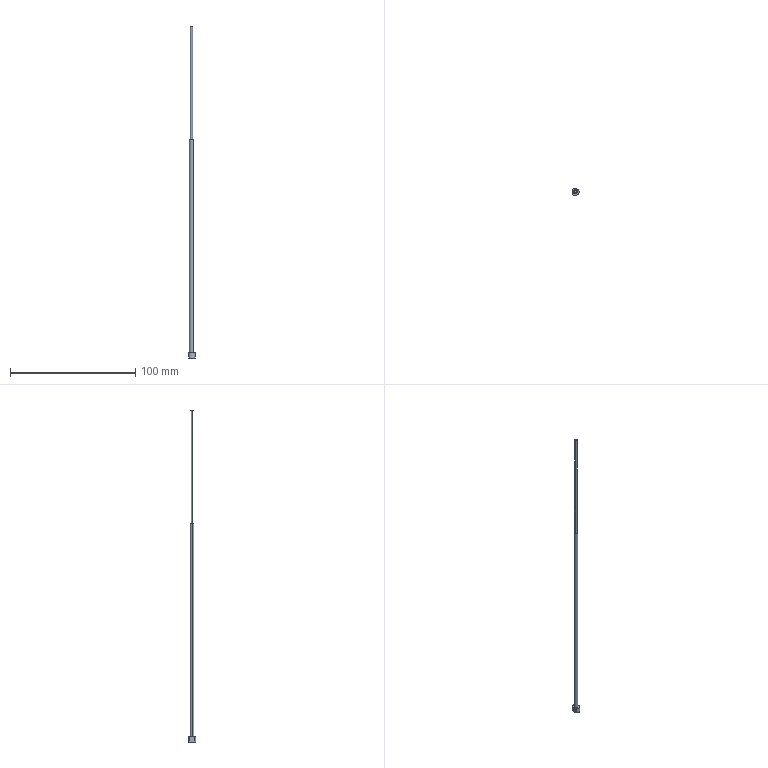Part | Creo | 1 solid | 10 faces | box 5 x 6 x 264.845 mm | volume 1588 mm3 | plane 5 | cylinder 5 | commonest cylinder face diameters 2 x2 3 x2 6 x1
STEP:
#1=CARTESIAN_POINT('',(-76.,0.,-292.));
#2=VERTEX_POINT('',#1);
#3=CARTESIAN_POINT('',(-81.,2.236,-292.));
#4=VERTEX_POINT('',#3);
#5=CARTESIAN_POINT('',(-79.,0.,-292.));
#6=DIRECTION('',(0.,0.,1.));
#7=DIRECTION('',(1.,0.,0.));
#8=AXIS2_PLACEMENT_3D('',#5,#6,#7);
#9=CIRCLE('',#8,3.);
#10=EDGE_CURVE('',#2,#4,#9,.T.);
#11=ORIENTED_EDGE('',*,*,#10,.F.);
#12=CARTESIAN_POINT('',(-81.,-2.236,-292.));
#13=VERTEX_POINT('',#12);
#14=CARTESIAN_POINT('',(-79.,0.,-292.));
#15=DIRECTION('',(0.,0.,1.));
#16=DIRECTION('',(-0.6667,-0.7454,0.));
#17=AXIS2_PLACEMENT_3D('',#14,#15,#16);
#18=CIRCLE('',#17,3.);
#19=EDGE_CURVE('',#13,#2,#18,.T.);
#20=ORIENTED_EDGE('',*,*,#19,.F.);
#21=CARTESIAN_POINT('',(-81.,-2.236,-292.));
#22=DIRECTION('',(0.,1.,0.));
#23=VECTOR('',#22,4.472);
#24=LINE('',#21,#23);
#25=EDGE_CURVE('',#13,#4,#24,.T.);
#26=ORIENTED_EDGE('',*,*,#25,.T.);
#27=EDGE_LOOP('',(#11,#20,#26));
#28=FACE_OUTER_BOUND('',#27,.F.);
#29=CARTESIAN_POINT('',(-77.5,0.,-292.));
#30=VERTEX_POINT('',#29);
#31=CARTESIAN_POINT('',(-80.5,0.,-292.));
#32=VERTEX_POINT('',#31);
#33=CARTESIAN_POINT('',(-79.,0.,-292.));
#34=DIRECTION('',(0.,0.,-1.));
#35=DIRECTION('',(1.,0.,0.));
#36=AXIS2_PLACEMENT_3D('',#33,#34,#35);
#37=CIRCLE('',#36,1.5);
#38=EDGE_CURVE('',#30,#32,#37,.T.);
#39=ORIENTED_EDGE('',*,*,#38,.F.);
#40=CARTESIAN_POINT('',(-79.,0.,-292.));
#41=DIRECTION('',(0.,0.,-1.));
#42=DIRECTION('',(-1.,0.,0.));
#43=AXIS2_PLACEMENT_3D('',#40,#41,#42);
#44=CIRCLE('',#43,1.5);
#45=EDGE_CURVE('',#32,#30,#44,.T.);
#46=ORIENTED_EDGE('',*,*,#45,.F.);
#47=EDGE_LOOP('',(#39,#46));
#48=FACE_BOUND('',#47,.F.);
#49=CARTESIAN_POINT('',(-79.,0.,-292.));
#50=DIRECTION('',(0.,0.,1.));
#51=DIRECTION('',(-1.,0.,0.));
#52=AXIS2_PLACEMENT_3D('',#49,#50,#51);
#53=PLANE('',#52);
#54=ADVANCED_FACE('',(#28,#48),#53,.T.);
#55=CARTESIAN_POINT('',(-80.5,0.,-122.));
#56=VERTEX_POINT('',#55);
#57=CARTESIAN_POINT('',(-77.5,0.,-122.));
#58=VERTEX_POINT('',#57);
#59=CARTESIAN_POINT('',(-79.,0.,-122.));
#60=DIRECTION('',(0.,0.,1.));
#61=DIRECTION('',(-1.,0.,0.));
#62=AXIS2_PLACEMENT_3D('',#59,#60,#61);
#63=CIRCLE('',#62,1.5);
#64=EDGE_CURVE('',#56,#58,#63,.T.);
#65=ORIENTED_EDGE('',*,*,#64,.T.);
#66=CARTESIAN_POINT('',(-77.5,0.,-122.));
#67=DIRECTION('',(0.,0.,-1.));
#68=VECTOR('',#67,170.);
#69=LINE('',#66,#68);
#70=EDGE_CURVE('',#58,#30,#69,.T.);
#71=ORIENTED_EDGE('',*,*,#70,.T.);
#72=ORIENTED_EDGE('',*,*,#38,.T.);
#73=CARTESIAN_POINT('',(-80.5,0.,-122.));
#74=DIRECTION('',(0.,0.,-1.));
#75=VECTOR('',#74,170.);
#76=LINE('',#73,#75);
#77=EDGE_CURVE('',#56,#32,#76,.T.);
#78=ORIENTED_EDGE('',*,*,#77,.F.);
#79=EDGE_LOOP('',(#65,#71,#72,#78));
#80=FACE_OUTER_BOUND('',#79,.F.);
#81=CARTESIAN_POINT('',(-79.,0.,-142.));
#82=DIRECTION('',(0.,0.,-1.));
#83=DIRECTION('',(1.,0.,0.));
#84=AXIS2_PLACEMENT_3D('',#81,#82,#83);
#85=CYLINDRICAL_SURFACE('',#84,1.5);
#86=ADVANCED_FACE('',(#80),#85,.T.);
#87=CARTESIAN_POINT('',(-79.,0.,-122.));
#88=DIRECTION('',(0.,0.,1.));
#89=DIRECTION('',(1.,0.,0.));
#90=AXIS2_PLACEMENT_3D('',#87,#88,#89);
#91=CIRCLE('',#90,1.5);
#92=EDGE_CURVE('',#58,#56,#91,.T.);
#93=ORIENTED_EDGE('',*,*,#92,.F.);
#94=ORIENTED_EDGE('',*,*,#64,.F.);
#95=EDGE_LOOP('',(#93,#94));
#96=FACE_OUTER_BOUND('',#95,.F.);
#97=CARTESIAN_POINT('',(-78.,0.,-122.));
#98=VERTEX_POINT('',#97);
#99=CARTESIAN_POINT('',(-80.,0.,-122.));
#100=VERTEX_POINT('',#99);
#101=CARTESIAN_POINT('',(-79.,0.,-122.));
#102=DIRECTION('',(0.,0.,-1.));
#103=DIRECTION('',(1.,0.,0.));
#104=AXIS2_PLACEMENT_3D('',#101,#102,#103);
#105=CIRCLE('',#104,1.);
#106=EDGE_CURVE('',#98,#100,#105,.T.);
#107=ORIENTED_EDGE('',*,*,#106,.F.);
#108=CARTESIAN_POINT('',(-79.,0.,-122.));
#109=DIRECTION('',(0.,0.,-1.));
#110=DIRECTION('',(-1.,0.,0.));
#111=AXIS2_PLACEMENT_3D('',#108,#109,#110);
#112=CIRCLE('',#111,1.);
#113=EDGE_CURVE('',#100,#98,#112,.T.);
#114=ORIENTED_EDGE('',*,*,#113,.F.);
#115=EDGE_LOOP('',(#107,#114));
#116=FACE_BOUND('',#115,.F.);
#117=CARTESIAN_POINT('',(-79.,0.,-122.));
#118=DIRECTION('',(0.,0.,1.));
#119=DIRECTION('',(-1.,0.,0.));
#120=AXIS2_PLACEMENT_3D('',#117,#118,#119);
#121=PLANE('',#120);
#122=ADVANCED_FACE('',(#96,#116),#121,.T.);
#123=ORIENTED_EDGE('',*,*,#106,.T.);
#124=CARTESIAN_POINT('',(-80.,0.,-31.155));
#125=VERTEX_POINT('',#124);
#126=CARTESIAN_POINT('',(-80.,0.,-31.155));
#127=DIRECTION('',(0.,0.,-1.));
#128=VECTOR('',#127,90.845);
#129=LINE('',#126,#128);
#130=EDGE_CURVE('',#125,#100,#129,.T.);
#131=ORIENTED_EDGE('',*,*,#130,.F.);
#132=CARTESIAN_POINT('',(-78.,0.,-31.155));
#133=VERTEX_POINT('',#132);
#134=CARTESIAN_POINT('',(-79.,0.,-31.155));
#135=DIRECTION('',(0.,0.,1.));
#136=DIRECTION('',(-1.,0.,0.));
#137=AXIS2_PLACEMENT_3D('',#134,#135,#136);
#138=CIRCLE('',#137,1.);
#139=EDGE_CURVE('',#125,#133,#138,.T.);
#140=ORIENTED_EDGE('',*,*,#139,.T.);
#141=CARTESIAN_POINT('',(-78.,0.,-31.155));
#142=DIRECTION('',(0.,0.,-1.));
#143=VECTOR('',#142,90.845);
#144=LINE('',#141,#143);
#145=EDGE_CURVE('',#133,#98,#144,.T.);
#146=ORIENTED_EDGE('',*,*,#145,.T.);
#147=EDGE_LOOP('',(#123,#131,#140,#146));
#148=FACE_OUTER_BOUND('',#147,.F.);
#149=CARTESIAN_POINT('',(-79.,0.,-24.));
#150=DIRECTION('',(0.,0.,-1.));
#151=DIRECTION('',(1.,0.,0.));
#152=AXIS2_PLACEMENT_3D('',#149,#150,#151);
#153=CYLINDRICAL_SURFACE('',#152,1.);
#154=ADVANCED_FACE('',(#148),#153,.T.);
#155=ORIENTED_EDGE('',*,*,#113,.T.);
#156=ORIENTED_EDGE('',*,*,#145,.F.);
#157=CARTESIAN_POINT('',(-79.,0.,-31.155));
#158=DIRECTION('',(0.,0.,1.));
#159=DIRECTION('',(1.,0.,0.));
#160=AXIS2_PLACEMENT_3D('',#157,#158,#159);
#161=CIRCLE('',#160,1.);
#162=EDGE_CURVE('',#133,#125,#161,.T.);
#163=ORIENTED_EDGE('',*,*,#162,.T.);
#164=ORIENTED_EDGE('',*,*,#130,.T.);
#165=EDGE_LOOP('',(#155,#156,#163,#164));
#166=FACE_OUTER_BOUND('',#165,.F.);
#167=CARTESIAN_POINT('',(-79.,0.,-24.));
#168=DIRECTION('',(0.,0.,-1.));
#169=DIRECTION('',(1.,0.,0.));
#170=AXIS2_PLACEMENT_3D('',#167,#168,#169);
#171=CYLINDRICAL_SURFACE('',#170,1.);
#172=ADVANCED_FACE('',(#166),#171,.T.);
#173=ORIENTED_EDGE('',*,*,#162,.F.);
#174=ORIENTED_EDGE('',*,*,#139,.F.);
#175=EDGE_LOOP('',(#173,#174));
#176=FACE_OUTER_BOUND('',#175,.F.);
#177=CARTESIAN_POINT('',(0.,0.,-31.155));
#178=DIRECTION('',(0.,0.,1.));
#179=DIRECTION('',(0.,1.,0.));
#180=AXIS2_PLACEMENT_3D('',#177,#178,#179);
#181=PLANE('',#180);
#182=ADVANCED_FACE('',(#176),#181,.T.);
#183=ORIENTED_EDGE('',*,*,#92,.T.);
#184=ORIENTED_EDGE('',*,*,#77,.T.);
#185=ORIENTED_EDGE('',*,*,#45,.T.);
#186=ORIENTED_EDGE('',*,*,#70,.F.);
#187=EDGE_LOOP('',(#183,#184,#185,#186));
#188=FACE_OUTER_BOUND('',#187,.F.);
#189=CARTESIAN_POINT('',(-79.,0.,-142.));
#190=DIRECTION('',(0.,0.,-1.));
#191=DIRECTION('',(1.,0.,0.));
#192=AXIS2_PLACEMENT_3D('',#189,#190,#191);
#193=CYLINDRICAL_SURFACE('',#192,1.5);
#194=ADVANCED_FACE('',(#188),#193,.T.);
#195=CARTESIAN_POINT('',(-81.,2.236,-296.));
#196=VERTEX_POINT('',#195);
#197=CARTESIAN_POINT('',(-81.,2.236,-296.));
#198=DIRECTION('',(0.,0.,1.));
#199=VECTOR('',#198,4.);
#200=LINE('',#197,#199);
#201=EDGE_CURVE('',#196,#4,#200,.T.);
#202=ORIENTED_EDGE('',*,*,#201,.F.);
#203=CARTESIAN_POINT('',(-76.,0.,-296.));
#204=VERTEX_POINT('',#203);
#205=CARTESIAN_POINT('',(-79.,0.,-296.));
#206=DIRECTION('',(0.,0.,-1.));
#207=DIRECTION('',(-0.6667,0.7454,0.));
#208=AXIS2_PLACEMENT_3D('',#205,#206,#207);
#209=CIRCLE('',#208,3.);
#210=EDGE_CURVE('',#196,#204,#209,.T.);
#211=ORIENTED_EDGE('',*,*,#210,.T.);
#212=CARTESIAN_POINT('',(-81.,-2.236,-296.));
#213=VERTEX_POINT('',#212);
#214=CARTESIAN_POINT('',(-79.,0.,-296.));
#215=DIRECTION('',(0.,0.,-1.));
#216=DIRECTION('',(1.,0.,0.));
#217=AXIS2_PLACEMENT_3D('',#214,#215,#216);
#218=CIRCLE('',#217,3.);
#219=EDGE_CURVE('',#204,#213,#218,.T.);
#220=ORIENTED_EDGE('',*,*,#219,.T.);
#221=CARTESIAN_POINT('',(-81.,-2.236,-292.));
#222=DIRECTION('',(0.,0.,-1.));
#223=VECTOR('',#222,4.);
#224=LINE('',#221,#223);
#225=EDGE_CURVE('',#13,#213,#224,.T.);
#226=ORIENTED_EDGE('',*,*,#225,.F.);
#227=ORIENTED_EDGE('',*,*,#19,.T.);
#228=ORIENTED_EDGE('',*,*,#10,.T.);
#229=EDGE_LOOP('',(#202,#211,#220,#226,#227,#228));
#230=FACE_OUTER_BOUND('',#229,.F.);
#231=CARTESIAN_POINT('',(-79.,0.,-296.));
#232=DIRECTION('',(0.,0.,1.));
#233=DIRECTION('',(-1.,0.,0.));
#234=AXIS2_PLACEMENT_3D('',#231,#232,#233);
#235=CYLINDRICAL_SURFACE('',#234,3.);
#236=ADVANCED_FACE('',(#230),#235,.T.);
#237=ORIENTED_EDGE('',*,*,#201,.T.);
#238=ORIENTED_EDGE('',*,*,#25,.F.);
#239=ORIENTED_EDGE('',*,*,#225,.T.);
#240=CARTESIAN_POINT('',(-81.,2.236,-296.));
#241=DIRECTION('',(0.,-1.,0.));
#242=VECTOR('',#241,4.472);
#243=LINE('',#240,#242);
#244=EDGE_CURVE('',#196,#213,#243,.T.);
#245=ORIENTED_EDGE('',*,*,#244,.F.);
#246=EDGE_LOOP('',(#237,#238,#239,#245));
#247=FACE_OUTER_BOUND('',#246,.F.);
#248=CARTESIAN_POINT('',(-81.,0.,-296.));
#249=DIRECTION('',(1.,0.,0.));
#250=DIRECTION('',(0.,0.,1.));
#251=AXIS2_PLACEMENT_3D('',#248,#249,#250);
#252=PLANE('',#251);
#253=ADVANCED_FACE('',(#247),#252,.F.);
#254=ORIENTED_EDGE('',*,*,#219,.F.);
#255=ORIENTED_EDGE('',*,*,#210,.F.);
#256=ORIENTED_EDGE('',*,*,#244,.T.);
#257=EDGE_LOOP('',(#254,#255,#256));
#258=FACE_OUTER_BOUND('',#257,.F.);
#259=CARTESIAN_POINT('',(-79.,0.,-296.));
#260=DIRECTION('',(0.,0.,-1.));
#261=DIRECTION('',(1.,0.,0.));
#262=AXIS2_PLACEMENT_3D('',#259,#260,#261);
#263=PLANE('',#262);
#264=ADVANCED_FACE('',(#258),#263,.T.);
#265=CLOSED_SHELL('',(#54,#86,#122,#154,#172,#182,#194,#236,#253,#264));
#266=MANIFOLD_SOLID_BREP('',#265);
#267=(LENGTH_UNIT()NAMED_UNIT(*)SI_UNIT(.MILLI.,.METRE.));
#268=UNCERTAINTY_MEASURE_WITH_UNIT(LENGTH_MEASURE(0.02649),#267,'','');
#269=(NAMED_UNIT(*)PLANE_ANGLE_UNIT()SI_UNIT($,.RADIAN.));
#270=PLANE_ANGLE_MEASURE_WITH_UNIT(PLANE_ANGLE_MEASURE(0.01745),#269);
#271=(CONVERSION_BASED_UNIT('DEGREE',#270)NAMED_UNIT(*)PLANE_ANGLE_UNIT());
#272=(NAMED_UNIT(*)SI_UNIT($,.STERADIAN.)SOLID_ANGLE_UNIT());
#273=(GEOMETRIC_REPRESENTATION_CONTEXT(3)GLOBAL_UNCERTAINTY_ASSIGNED_CONTEXT((#268))GLOBAL_UNIT_ASSIGNED_CONTEXT((#267,#271,#272))REPRESENTATION_CONTEXT('',''));
#274=ADVANCED_BREP_SHAPE_REPRESENTATION('',(#266),#273);